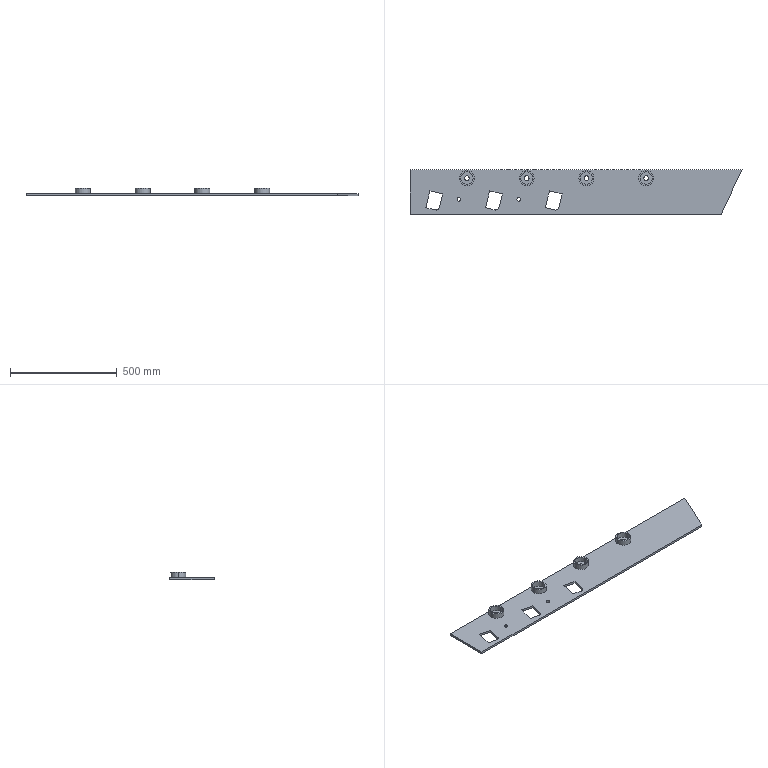Part | STEP file | Edge plate 1_Default<As machined> | 5 solids | 57 faces | box 1555 x 210 x 35 mm | volume 3116927 mm3 | cylinder 31 | plane 26 | commonest cylinder face diameters 22 x8 58 x8 70 x8 17 x4 30 x3